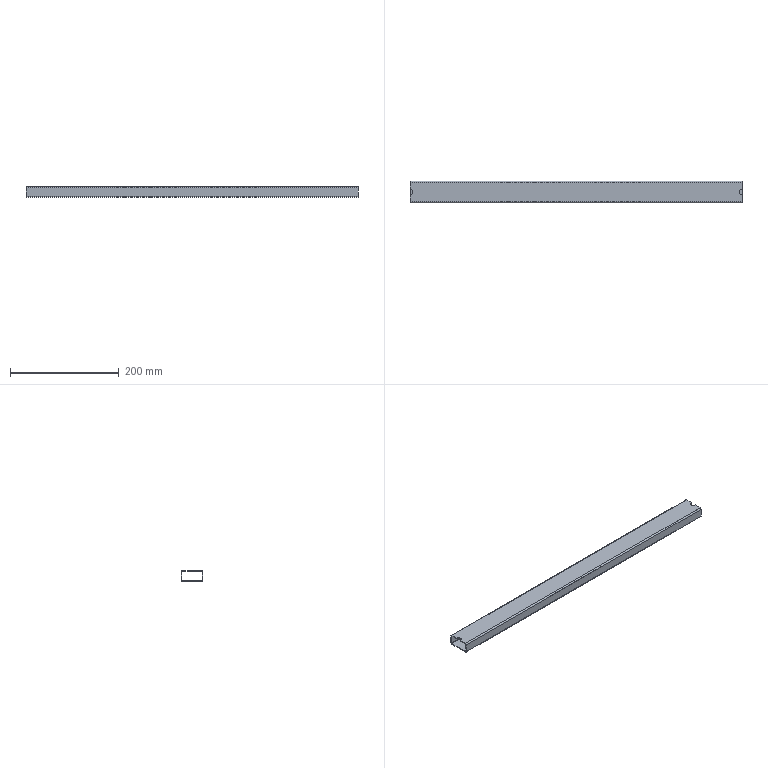Part | STEP file | Q7C0505 | 1 solid | 20 faces | box 610 x 40 x 20 mm | volume 101443 mm3 | plane 10 | cylinder 10 | commonest cylinder face diameters 2 x4 5 x4 10 x2